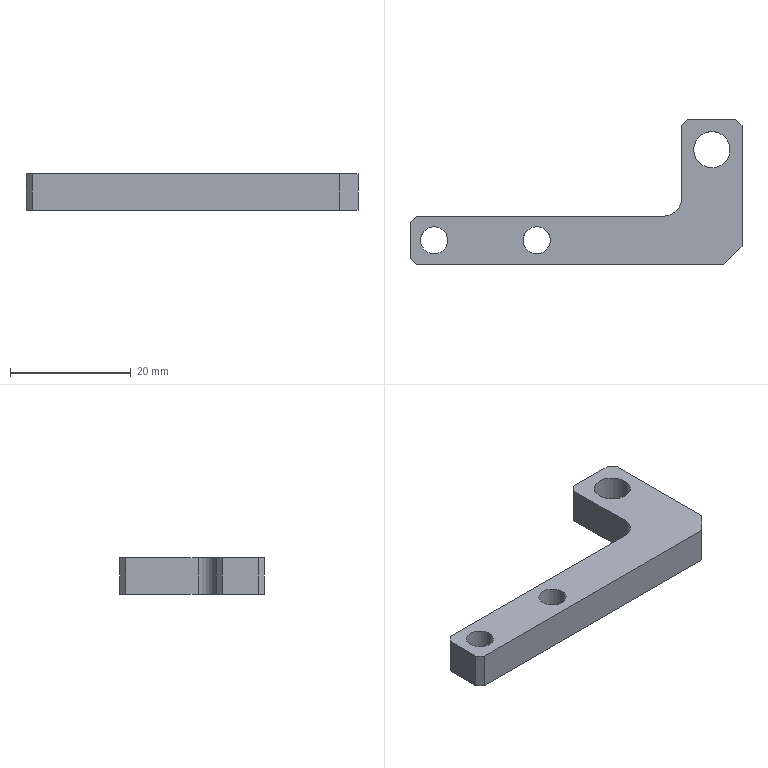Part | SolidWorks | features Chamfer 2, Extrusion 1, Fillet 1 | 1 solid | 20 faces | box 55 x 24 x 6 mm | volume 3212 mm3 | plane 13 | cylinder 7 | commonest cylinder face diameters 4.5 x4 6 x3
STEP:
#1=CARTESIAN_POINT('',(-8.,19.,3.));
#2=VERTEX_POINT('',#1);
#3=CARTESIAN_POINT('',(-2.,19.,3.));
#4=VERTEX_POINT('',#3);
#5=CARTESIAN_POINT('',(-5.,19.,3.));
#6=DIRECTION('',(0.,0.,1.));
#7=DIRECTION('',(1.,0.,0.));
#8=AXIS2_PLACEMENT_3D('',#5,#6,#7);
#9=CIRCLE('',#8,3.);
#10=EDGE_CURVE('',#2,#4,#9,.T.);
#11=ORIENTED_EDGE('',*,*,#10,.T.);
#12=CARTESIAN_POINT('',(-2.,19.,-3.));
#13=VERTEX_POINT('',#12);
#14=CARTESIAN_POINT('',(-2.,19.,3.));
#15=DIRECTION('',(0.,0.,-1.));
#16=VECTOR('',#15,1000.);
#17=LINE('',#14,#16);
#18=EDGE_CURVE('',#4,#13,#17,.T.);
#19=ORIENTED_EDGE('',*,*,#18,.T.);
#20=CARTESIAN_POINT('',(-8.,19.,-3.));
#21=VERTEX_POINT('',#20);
#22=CARTESIAN_POINT('',(-5.,19.,-3.));
#23=DIRECTION('',(0.,0.,1.));
#24=DIRECTION('',(1.,0.,0.));
#25=AXIS2_PLACEMENT_3D('',#22,#23,#24);
#26=CIRCLE('',#25,3.);
#27=EDGE_CURVE('',#21,#13,#26,.T.);
#28=ORIENTED_EDGE('',*,*,#27,.F.);
#29=CARTESIAN_POINT('',(-8.,19.,3.));
#30=DIRECTION('',(0.,0.,-1.));
#31=VECTOR('',#30,1000.);
#32=LINE('',#29,#31);
#33=EDGE_CURVE('',#2,#21,#32,.T.);
#34=ORIENTED_EDGE('',*,*,#33,.F.);
#35=EDGE_LOOP('',(#11,#19,#28,#34));
#36=FACE_OUTER_BOUND('',#35,.T.);
#37=CARTESIAN_POINT('',(-5.,19.,3.));
#38=DIRECTION('',(0.,0.,-1.));
#39=DIRECTION('',(-1.,0.,0.));
#40=AXIS2_PLACEMENT_3D('',#37,#38,#39);
#41=CYLINDRICAL_SURFACE('',#40,3.);
#42=ADVANCED_FACE('',(#36),#41,.F.);
#43=CARTESIAN_POINT('',(-36.25,4.,3.));
#44=VERTEX_POINT('',#43);
#45=CARTESIAN_POINT('',(-31.75,4.,3.));
#46=VERTEX_POINT('',#45);
#47=CARTESIAN_POINT('',(-34.,4.,3.));
#48=DIRECTION('',(0.,0.,1.));
#49=DIRECTION('',(1.,0.,0.));
#50=AXIS2_PLACEMENT_3D('',#47,#48,#49);
#51=CIRCLE('',#50,2.25);
#52=EDGE_CURVE('',#44,#46,#51,.T.);
#53=ORIENTED_EDGE('',*,*,#52,.T.);
#54=CARTESIAN_POINT('',(-31.75,4.,-3.));
#55=VERTEX_POINT('',#54);
#56=CARTESIAN_POINT('',(-31.75,4.,3.));
#57=DIRECTION('',(0.,0.,-1.));
#58=VECTOR('',#57,1000.);
#59=LINE('',#56,#58);
#60=EDGE_CURVE('',#46,#55,#59,.T.);
#61=ORIENTED_EDGE('',*,*,#60,.T.);
#62=CARTESIAN_POINT('',(-36.25,4.,-3.));
#63=VERTEX_POINT('',#62);
#64=CARTESIAN_POINT('',(-34.,4.,-3.));
#65=DIRECTION('',(0.,0.,1.));
#66=DIRECTION('',(1.,0.,0.));
#67=AXIS2_PLACEMENT_3D('',#64,#65,#66);
#68=CIRCLE('',#67,2.25);
#69=EDGE_CURVE('',#63,#55,#68,.T.);
#70=ORIENTED_EDGE('',*,*,#69,.F.);
#71=CARTESIAN_POINT('',(-36.25,4.,3.));
#72=DIRECTION('',(0.,0.,-1.));
#73=VECTOR('',#72,1000.);
#74=LINE('',#71,#73);
#75=EDGE_CURVE('',#44,#63,#74,.T.);
#76=ORIENTED_EDGE('',*,*,#75,.F.);
#77=EDGE_LOOP('',(#53,#61,#70,#76));
#78=FACE_OUTER_BOUND('',#77,.T.);
#79=CARTESIAN_POINT('',(-34.,4.,3.));
#80=DIRECTION('',(0.,0.,-1.));
#81=DIRECTION('',(-1.,0.,0.));
#82=AXIS2_PLACEMENT_3D('',#79,#80,#81);
#83=CYLINDRICAL_SURFACE('',#82,2.25);
#84=ADVANCED_FACE('',(#78),#83,.F.);
#85=CARTESIAN_POINT('',(-53.25,4.,3.));
#86=VERTEX_POINT('',#85);
#87=CARTESIAN_POINT('',(-48.75,4.,3.));
#88=VERTEX_POINT('',#87);
#89=CARTESIAN_POINT('',(-51.,4.,3.));
#90=DIRECTION('',(0.,0.,1.));
#91=DIRECTION('',(1.,0.,0.));
#92=AXIS2_PLACEMENT_3D('',#89,#90,#91);
#93=CIRCLE('',#92,2.25);
#94=EDGE_CURVE('',#86,#88,#93,.T.);
#95=ORIENTED_EDGE('',*,*,#94,.T.);
#96=CARTESIAN_POINT('',(-48.75,4.,-3.));
#97=VERTEX_POINT('',#96);
#98=CARTESIAN_POINT('',(-48.75,4.,3.));
#99=DIRECTION('',(0.,0.,-1.));
#100=VECTOR('',#99,1000.);
#101=LINE('',#98,#100);
#102=EDGE_CURVE('',#88,#97,#101,.T.);
#103=ORIENTED_EDGE('',*,*,#102,.T.);
#104=CARTESIAN_POINT('',(-53.25,4.,-3.));
#105=VERTEX_POINT('',#104);
#106=CARTESIAN_POINT('',(-51.,4.,-3.));
#107=DIRECTION('',(0.,0.,1.));
#108=DIRECTION('',(1.,0.,0.));
#109=AXIS2_PLACEMENT_3D('',#106,#107,#108);
#110=CIRCLE('',#109,2.25);
#111=EDGE_CURVE('',#105,#97,#110,.T.);
#112=ORIENTED_EDGE('',*,*,#111,.F.);
#113=CARTESIAN_POINT('',(-53.25,4.,3.));
#114=DIRECTION('',(0.,0.,-1.));
#115=VECTOR('',#114,1000.);
#116=LINE('',#113,#115);
#117=EDGE_CURVE('',#86,#105,#116,.T.);
#118=ORIENTED_EDGE('',*,*,#117,.F.);
#119=EDGE_LOOP('',(#95,#103,#112,#118));
#120=FACE_OUTER_BOUND('',#119,.T.);
#121=CARTESIAN_POINT('',(-51.,4.,3.));
#122=DIRECTION('',(0.,0.,-1.));
#123=DIRECTION('',(-1.,0.,0.));
#124=AXIS2_PLACEMENT_3D('',#121,#122,#123);
#125=CYLINDRICAL_SURFACE('',#124,2.25);
#126=ADVANCED_FACE('',(#120),#125,.F.);
#127=ORIENTED_EDGE('',*,*,#52,.F.);
#128=CARTESIAN_POINT('',(-34.,4.,3.));
#129=DIRECTION('',(0.,0.,1.));
#130=DIRECTION('',(1.,0.,0.));
#131=AXIS2_PLACEMENT_3D('',#128,#129,#130);
#132=CIRCLE('',#131,2.25);
#133=EDGE_CURVE('',#46,#44,#132,.T.);
#134=ORIENTED_EDGE('',*,*,#133,.F.);
#135=EDGE_LOOP('',(#127,#134));
#136=FACE_BOUND('',#135,.T.);
#137=CARTESIAN_POINT('',(-55.,7.,3.));
#138=VERTEX_POINT('',#137);
#139=CARTESIAN_POINT('',(-55.,1.,3.));
#140=VERTEX_POINT('',#139);
#141=CARTESIAN_POINT('',(-55.,0.,3.));
#142=DIRECTION('',(0.,-1.,0.));
#143=VECTOR('',#142,1000.);
#144=LINE('',#141,#143);
#145=EDGE_CURVE('',#138,#140,#144,.T.);
#146=ORIENTED_EDGE('',*,*,#145,.T.);
#147=CARTESIAN_POINT('',(-54.,0.,3.));
#148=VERTEX_POINT('',#147);
#149=CARTESIAN_POINT('',(-39.,-15.,3.));
#150=DIRECTION('',(0.7071,-0.7071,0.));
#151=VECTOR('',#150,1000.);
#152=LINE('',#149,#151);
#153=EDGE_CURVE('',#140,#148,#152,.T.);
#154=ORIENTED_EDGE('',*,*,#153,.T.);
#155=CARTESIAN_POINT('',(-3.,0.,3.));
#156=VERTEX_POINT('',#155);
#157=CARTESIAN_POINT('',(0.,0.,3.));
#158=DIRECTION('',(1.,0.,0.));
#159=VECTOR('',#158,1000.);
#160=LINE('',#157,#159);
#161=EDGE_CURVE('',#148,#156,#160,.T.);
#162=ORIENTED_EDGE('',*,*,#161,.T.);
#163=CARTESIAN_POINT('',(0.,3.,3.));
#164=VERTEX_POINT('',#163);
#165=CARTESIAN_POINT('',(10.5,13.5,3.));
#166=DIRECTION('',(0.7071,0.7071,0.));
#167=VECTOR('',#166,1000.);
#168=LINE('',#165,#167);
#169=EDGE_CURVE('',#156,#164,#168,.T.);
#170=ORIENTED_EDGE('',*,*,#169,.T.);
#171=CARTESIAN_POINT('',(0.,23.,3.));
#172=VERTEX_POINT('',#171);
#173=CARTESIAN_POINT('',(0.,0.,3.));
#174=DIRECTION('',(0.,1.,0.));
#175=VECTOR('',#174,1000.);
#176=LINE('',#173,#175);
#177=EDGE_CURVE('',#164,#172,#176,.T.);
#178=ORIENTED_EDGE('',*,*,#177,.T.);
#179=CARTESIAN_POINT('',(-1.,24.,3.));
#180=VERTEX_POINT('',#179);
#181=CARTESIAN_POINT('',(-0.5,23.5,3.));
#182=DIRECTION('',(-0.7071,0.7071,0.));
#183=VECTOR('',#182,1000.);
#184=LINE('',#181,#183);
#185=EDGE_CURVE('',#172,#180,#184,.T.);
#186=ORIENTED_EDGE('',*,*,#185,.T.);
#187=CARTESIAN_POINT('',(-9.,24.,3.));
#188=VERTEX_POINT('',#187);
#189=CARTESIAN_POINT('',(0.,24.,3.));
#190=DIRECTION('',(-1.,0.,0.));
#191=VECTOR('',#190,1000.);
#192=LINE('',#189,#191);
#193=EDGE_CURVE('',#180,#188,#192,.T.);
#194=ORIENTED_EDGE('',*,*,#193,.T.);
#195=CARTESIAN_POINT('',(-10.,23.,3.));
#196=VERTEX_POINT('',#195);
#197=CARTESIAN_POINT('',(-4.5,28.5,3.));
#198=DIRECTION('',(-0.7071,-0.7071,0.));
#199=VECTOR('',#198,1000.);
#200=LINE('',#197,#199);
#201=EDGE_CURVE('',#188,#196,#200,.T.);
#202=ORIENTED_EDGE('',*,*,#201,.T.);
#203=CARTESIAN_POINT('',(-10.,11.,3.));
#204=VERTEX_POINT('',#203);
#205=CARTESIAN_POINT('',(-10.,24.,3.));
#206=DIRECTION('',(0.,-1.,0.));
#207=VECTOR('',#206,1000.);
#208=LINE('',#205,#207);
#209=EDGE_CURVE('',#196,#204,#208,.T.);
#210=ORIENTED_EDGE('',*,*,#209,.T.);
#211=CARTESIAN_POINT('',(-13.,8.,3.));
#212=VERTEX_POINT('',#211);
#213=CARTESIAN_POINT('',(-13.,11.,3.));
#214=DIRECTION('',(0.,0.,-1.));
#215=DIRECTION('',(1.,0.,0.));
#216=AXIS2_PLACEMENT_3D('',#213,#214,#215);
#217=CIRCLE('',#216,3.);
#218=EDGE_CURVE('',#204,#212,#217,.T.);
#219=ORIENTED_EDGE('',*,*,#218,.T.);
#220=CARTESIAN_POINT('',(-54.,8.,3.));
#221=VERTEX_POINT('',#220);
#222=CARTESIAN_POINT('',(-55.,8.,3.));
#223=DIRECTION('',(-1.,0.,0.));
#224=VECTOR('',#223,1000.);
#225=LINE('',#222,#224);
#226=EDGE_CURVE('',#212,#221,#225,.T.);
#227=ORIENTED_EDGE('',*,*,#226,.T.);
#228=CARTESIAN_POINT('',(-19.,43.,3.));
#229=DIRECTION('',(-0.7071,-0.7071,0.));
#230=VECTOR('',#229,1000.);
#231=LINE('',#228,#230);
#232=EDGE_CURVE('',#221,#138,#231,.T.);
#233=ORIENTED_EDGE('',*,*,#232,.T.);
#234=EDGE_LOOP('',(#146,#154,#162,#170,#178,#186,#194,#202,#210,#219,#227,#233));
#235=FACE_OUTER_BOUND('',#234,.T.);
#236=ORIENTED_EDGE('',*,*,#94,.F.);
#237=CARTESIAN_POINT('',(-51.,4.,3.));
#238=DIRECTION('',(0.,0.,1.));
#239=DIRECTION('',(1.,0.,0.));
#240=AXIS2_PLACEMENT_3D('',#237,#238,#239);
#241=CIRCLE('',#240,2.25);
#242=EDGE_CURVE('',#88,#86,#241,.T.);
#243=ORIENTED_EDGE('',*,*,#242,.F.);
#244=EDGE_LOOP('',(#236,#243));
#245=FACE_BOUND('',#244,.T.);
#246=ORIENTED_EDGE('',*,*,#10,.F.);
#247=CARTESIAN_POINT('',(-5.,19.,3.));
#248=DIRECTION('',(0.,0.,1.));
#249=DIRECTION('',(1.,0.,0.));
#250=AXIS2_PLACEMENT_3D('',#247,#248,#249);
#251=CIRCLE('',#250,3.);
#252=EDGE_CURVE('',#4,#2,#251,.T.);
#253=ORIENTED_EDGE('',*,*,#252,.F.);
#254=EDGE_LOOP('',(#246,#253));
#255=FACE_BOUND('',#254,.T.);
#256=CARTESIAN_POINT('',(0.,24.,3.));
#257=DIRECTION('',(0.,0.,1.));
#258=DIRECTION('',(1.,0.,0.));
#259=AXIS2_PLACEMENT_3D('',#256,#257,#258);
#260=PLANE('',#259);
#261=ADVANCED_FACE('',(#136,#235,#245,#255),#260,.T.);
#262=ORIENTED_EDGE('',*,*,#69,.T.);
#263=CARTESIAN_POINT('',(-34.,4.,-3.));
#264=DIRECTION('',(0.,0.,1.));
#265=DIRECTION('',(1.,0.,0.));
#266=AXIS2_PLACEMENT_3D('',#263,#264,#265);
#267=CIRCLE('',#266,2.25);
#268=EDGE_CURVE('',#55,#63,#267,.T.);
#269=ORIENTED_EDGE('',*,*,#268,.T.);
#270=EDGE_LOOP('',(#262,#269));
#271=FACE_BOUND('',#270,.T.);
#272=CARTESIAN_POINT('',(-54.,0.,-3.));
#273=VERTEX_POINT('',#272);
#274=CARTESIAN_POINT('',(-3.,0.,-3.));
#275=VERTEX_POINT('',#274);
#276=CARTESIAN_POINT('',(0.,0.,-3.));
#277=DIRECTION('',(1.,0.,0.));
#278=VECTOR('',#277,1000.);
#279=LINE('',#276,#278);
#280=EDGE_CURVE('',#273,#275,#279,.T.);
#281=ORIENTED_EDGE('',*,*,#280,.F.);
#282=CARTESIAN_POINT('',(-55.,1.,-3.));
#283=VERTEX_POINT('',#282);
#284=CARTESIAN_POINT('',(-54.,0.,-3.));
#285=DIRECTION('',(-0.7071,0.7071,0.));
#286=VECTOR('',#285,1000.);
#287=LINE('',#284,#286);
#288=EDGE_CURVE('',#273,#283,#287,.T.);
#289=ORIENTED_EDGE('',*,*,#288,.T.);
#290=CARTESIAN_POINT('',(-55.,7.,-3.));
#291=VERTEX_POINT('',#290);
#292=CARTESIAN_POINT('',(-55.,0.,-3.));
#293=DIRECTION('',(0.,-1.,0.));
#294=VECTOR('',#293,1000.);
#295=LINE('',#292,#294);
#296=EDGE_CURVE('',#291,#283,#295,.T.);
#297=ORIENTED_EDGE('',*,*,#296,.F.);
#298=CARTESIAN_POINT('',(-54.,8.,-3.));
#299=VERTEX_POINT('',#298);
#300=CARTESIAN_POINT('',(-55.,7.,-3.));
#301=DIRECTION('',(0.7071,0.7071,0.));
#302=VECTOR('',#301,1000.);
#303=LINE('',#300,#302);
#304=EDGE_CURVE('',#291,#299,#303,.T.);
#305=ORIENTED_EDGE('',*,*,#304,.T.);
#306=CARTESIAN_POINT('',(-13.,8.,-3.));
#307=VERTEX_POINT('',#306);
#308=CARTESIAN_POINT('',(-55.,8.,-3.));
#309=DIRECTION('',(-1.,0.,0.));
#310=VECTOR('',#309,1000.);
#311=LINE('',#308,#310);
#312=EDGE_CURVE('',#307,#299,#311,.T.);
#313=ORIENTED_EDGE('',*,*,#312,.F.);
#314=CARTESIAN_POINT('',(-10.,11.,-3.));
#315=VERTEX_POINT('',#314);
#316=CARTESIAN_POINT('',(-13.,11.,-3.));
#317=DIRECTION('',(0.,0.,1.));
#318=DIRECTION('',(1.,0.,0.));
#319=AXIS2_PLACEMENT_3D('',#316,#317,#318);
#320=CIRCLE('',#319,3.);
#321=EDGE_CURVE('',#307,#315,#320,.T.);
#322=ORIENTED_EDGE('',*,*,#321,.T.);
#323=CARTESIAN_POINT('',(-10.,23.,-3.));
#324=VERTEX_POINT('',#323);
#325=CARTESIAN_POINT('',(-10.,24.,-3.));
#326=DIRECTION('',(0.,-1.,0.));
#327=VECTOR('',#326,1000.);
#328=LINE('',#325,#327);
#329=EDGE_CURVE('',#324,#315,#328,.T.);
#330=ORIENTED_EDGE('',*,*,#329,.F.);
#331=CARTESIAN_POINT('',(-9.,24.,-3.));
#332=VERTEX_POINT('',#331);
#333=CARTESIAN_POINT('',(-10.,23.,-3.));
#334=DIRECTION('',(0.7071,0.7071,0.));
#335=VECTOR('',#334,1000.);
#336=LINE('',#333,#335);
#337=EDGE_CURVE('',#324,#332,#336,.T.);
#338=ORIENTED_EDGE('',*,*,#337,.T.);
#339=CARTESIAN_POINT('',(-1.,24.,-3.));
#340=VERTEX_POINT('',#339);
#341=CARTESIAN_POINT('',(0.,24.,-3.));
#342=DIRECTION('',(-1.,0.,0.));
#343=VECTOR('',#342,1000.);
#344=LINE('',#341,#343);
#345=EDGE_CURVE('',#340,#332,#344,.T.);
#346=ORIENTED_EDGE('',*,*,#345,.F.);
#347=CARTESIAN_POINT('',(0.,23.,-3.));
#348=VERTEX_POINT('',#347);
#349=CARTESIAN_POINT('',(-1.,24.,-3.));
#350=DIRECTION('',(0.7071,-0.7071,0.));
#351=VECTOR('',#350,1000.);
#352=LINE('',#349,#351);
#353=EDGE_CURVE('',#340,#348,#352,.T.);
#354=ORIENTED_EDGE('',*,*,#353,.T.);
#355=CARTESIAN_POINT('',(0.,3.,-3.));
#356=VERTEX_POINT('',#355);
#357=CARTESIAN_POINT('',(0.,0.,-3.));
#358=DIRECTION('',(0.,1.,0.));
#359=VECTOR('',#358,1000.);
#360=LINE('',#357,#359);
#361=EDGE_CURVE('',#356,#348,#360,.T.);
#362=ORIENTED_EDGE('',*,*,#361,.F.);
#363=CARTESIAN_POINT('',(0.,3.,-3.));
#364=DIRECTION('',(-0.7071,-0.7071,0.));
#365=VECTOR('',#364,1000.);
#366=LINE('',#363,#365);
#367=EDGE_CURVE('',#356,#275,#366,.T.);
#368=ORIENTED_EDGE('',*,*,#367,.T.);
#369=EDGE_LOOP('',(#281,#289,#297,#305,#313,#322,#330,#338,#346,#354,#362,#368));
#370=FACE_OUTER_BOUND('',#369,.T.);
#371=ORIENTED_EDGE('',*,*,#111,.T.);
#372=CARTESIAN_POINT('',(-51.,4.,-3.));
#373=DIRECTION('',(0.,0.,1.));
#374=DIRECTION('',(1.,0.,0.));
#375=AXIS2_PLACEMENT_3D('',#372,#373,#374);
#376=CIRCLE('',#375,2.25);
#377=EDGE_CURVE('',#97,#105,#376,.T.);
#378=ORIENTED_EDGE('',*,*,#377,.T.);
#379=EDGE_LOOP('',(#371,#378));
#380=FACE_BOUND('',#379,.T.);
#381=ORIENTED_EDGE('',*,*,#27,.T.);
#382=CARTESIAN_POINT('',(-5.,19.,-3.));
#383=DIRECTION('',(0.,0.,1.));
#384=DIRECTION('',(1.,0.,0.));
#385=AXIS2_PLACEMENT_3D('',#382,#383,#384);
#386=CIRCLE('',#385,3.);
#387=EDGE_CURVE('',#13,#21,#386,.T.);
#388=ORIENTED_EDGE('',*,*,#387,.T.);
#389=EDGE_LOOP('',(#381,#388));
#390=FACE_BOUND('',#389,.T.);
#391=CARTESIAN_POINT('',(0.,24.,-3.));
#392=DIRECTION('',(0.,0.,1.));
#393=DIRECTION('',(1.,0.,0.));
#394=AXIS2_PLACEMENT_3D('',#391,#392,#393);
#395=PLANE('',#394);
#396=ADVANCED_FACE('',(#271,#370,#380,#390),#395,.F.);
#397=ORIENTED_EDGE('',*,*,#361,.T.);
#398=CARTESIAN_POINT('',(0.,23.,3.));
#399=DIRECTION('',(0.,0.,1.));
#400=VECTOR('',#399,1000.);
#401=LINE('',#398,#400);
#402=EDGE_CURVE('',#348,#172,#401,.T.);
#403=ORIENTED_EDGE('',*,*,#402,.T.);
#404=ORIENTED_EDGE('',*,*,#177,.F.);
#405=CARTESIAN_POINT('',(0.,3.,3.));
#406=DIRECTION('',(0.,0.,-1.));
#407=VECTOR('',#406,1000.);
#408=LINE('',#405,#407);
#409=EDGE_CURVE('',#164,#356,#408,.T.);
#410=ORIENTED_EDGE('',*,*,#409,.T.);
#411=EDGE_LOOP('',(#397,#403,#404,#410));
#412=FACE_OUTER_BOUND('',#411,.T.);
#413=CARTESIAN_POINT('',(0.,0.,3.));
#414=DIRECTION('',(-1.,0.,0.));
#415=DIRECTION('',(0.,0.,1.));
#416=AXIS2_PLACEMENT_3D('',#413,#414,#415);
#417=PLANE('',#416);
#418=ADVANCED_FACE('',(#412),#417,.F.);
#419=ORIENTED_EDGE('',*,*,#345,.T.);
#420=CARTESIAN_POINT('',(-9.,24.,3.));
#421=DIRECTION('',(0.,0.,1.));
#422=VECTOR('',#421,1000.);
#423=LINE('',#420,#422);
#424=EDGE_CURVE('',#332,#188,#423,.T.);
#425=ORIENTED_EDGE('',*,*,#424,.T.);
#426=ORIENTED_EDGE('',*,*,#193,.F.);
#427=CARTESIAN_POINT('',(-1.,24.,3.));
#428=DIRECTION('',(0.,0.,-1.));
#429=VECTOR('',#428,1000.);
#430=LINE('',#427,#429);
#431=EDGE_CURVE('',#180,#340,#430,.T.);
#432=ORIENTED_EDGE('',*,*,#431,.T.);
#433=EDGE_LOOP('',(#419,#425,#426,#432));
#434=FACE_OUTER_BOUND('',#433,.T.);
#435=CARTESIAN_POINT('',(0.,24.,3.));
#436=DIRECTION('',(0.,-1.,0.));
#437=DIRECTION('',(0.,0.,-1.));
#438=AXIS2_PLACEMENT_3D('',#435,#436,#437);
#439=PLANE('',#438);
#440=ADVANCED_FACE('',(#434),#439,.F.);
#441=ORIENTED_EDGE('',*,*,#209,.F.);
#442=CARTESIAN_POINT('',(-10.,23.,3.));
#443=DIRECTION('',(0.,0.,-1.));
#444=VECTOR('',#443,1000.);
#445=LINE('',#442,#444);
#446=EDGE_CURVE('',#196,#324,#445,.T.);
#447=ORIENTED_EDGE('',*,*,#446,.T.);
#448=ORIENTED_EDGE('',*,*,#329,.T.);
#449=CARTESIAN_POINT('',(-10.,11.,3.));
#450=DIRECTION('',(0.,0.,1.));
#451=VECTOR('',#450,1000.);
#452=LINE('',#449,#451);
#453=EDGE_CURVE('',#315,#204,#452,.T.);
#454=ORIENTED_EDGE('',*,*,#453,.T.);
#455=EDGE_LOOP('',(#441,#447,#448,#454));
#456=FACE_OUTER_BOUND('',#455,.T.);
#457=CARTESIAN_POINT('',(-10.,24.,3.));
#458=DIRECTION('',(1.,0.,0.));
#459=DIRECTION('',(0.,1.,0.));
#460=AXIS2_PLACEMENT_3D('',#457,#458,#459);
#461=PLANE('',#460);
#462=ADVANCED_FACE('',(#456),#461,.F.);
#463=ORIENTED_EDGE('',*,*,#312,.T.);
#464=CARTESIAN_POINT('',(-54.,8.,3.));
#465=DIRECTION('',(0.,0.,1.));
#466=VECTOR('',#465,1000.);
#467=LINE('',#464,#466);
#468=EDGE_CURVE('',#299,#221,#467,.T.);
#469=ORIENTED_EDGE('',*,*,#468,.T.);
#470=ORIENTED_EDGE('',*,*,#226,.F.);
#471=CARTESIAN_POINT('',(-13.,8.,-3.));
#472=DIRECTION('',(0.,0.,-1.));
#473=VECTOR('',#472,1000.);
#474=LINE('',#471,#473);
#475=EDGE_CURVE('',#212,#307,#474,.T.);
#476=ORIENTED_EDGE('',*,*,#475,.T.);
#477=EDGE_LOOP('',(#463,#469,#470,#476));
#478=FACE_OUTER_BOUND('',#477,.T.);
#479=CARTESIAN_POINT('',(-55.,8.,3.));
#480=DIRECTION('',(0.,-1.,0.));
#481=DIRECTION('',(0.,0.,-1.));
#482=AXIS2_PLACEMENT_3D('',#479,#480,#481);
#483=PLANE('',#482);
#484=ADVANCED_FACE('',(#478),#483,.F.);
#485=ORIENTED_EDGE('',*,*,#296,.T.);
#486=CARTESIAN_POINT('',(-55.,1.,3.));
#487=DIRECTION('',(0.,0.,1.));
#488=VECTOR('',#487,1000.);
#489=LINE('',#486,#488);
#490=EDGE_CURVE('',#283,#140,#489,.T.);
#491=ORIENTED_EDGE('',*,*,#490,.T.);
#492=ORIENTED_EDGE('',*,*,#145,.F.);
#493=CARTESIAN_POINT('',(-55.,7.,3.));
#494=DIRECTION('',(0.,0.,-1.));
#495=VECTOR('',#494,1000.);
#496=LINE('',#493,#495);
#497=EDGE_CURVE('',#138,#291,#496,.T.);
#498=ORIENTED_EDGE('',*,*,#497,.T.);
#499=EDGE_LOOP('',(#485,#491,#492,#498));
#500=FACE_OUTER_BOUND('',#499,.T.);
#501=CARTESIAN_POINT('',(-55.,0.,3.));
#502=DIRECTION('',(1.,0.,0.));
#503=DIRECTION('',(0.,0.,-1.));
#504=AXIS2_PLACEMENT_3D('',#501,#502,#503);
#505=PLANE('',#504);
#506=ADVANCED_FACE('',(#500),#505,.F.);
#507=ORIENTED_EDGE('',*,*,#161,.F.);
#508=CARTESIAN_POINT('',(-54.,0.,3.));
#509=DIRECTION('',(0.,0.,-1.));
#510=VECTOR('',#509,1000.);
#511=LINE('',#508,#510);
#512=EDGE_CURVE('',#148,#273,#511,.T.);
#513=ORIENTED_EDGE('',*,*,#512,.T.);
#514=ORIENTED_EDGE('',*,*,#280,.T.);
#515=CARTESIAN_POINT('',(-3.,0.,3.));
#516=DIRECTION('',(0.,0.,1.));
#517=VECTOR('',#516,1000.);
#518=LINE('',#515,#517);
#519=EDGE_CURVE('',#275,#156,#518,.T.);
#520=ORIENTED_EDGE('',*,*,#519,.T.);
#521=EDGE_LOOP('',(#507,#513,#514,#520));
#522=FACE_OUTER_BOUND('',#521,.T.);
#523=CARTESIAN_POINT('',(0.,0.,3.));
#524=DIRECTION('',(0.,1.,0.));
#525=DIRECTION('',(-1.,0.,0.));
#526=AXIS2_PLACEMENT_3D('',#523,#524,#525);
#527=PLANE('',#526);
#528=ADVANCED_FACE('',(#522),#527,.F.);
#529=ORIENTED_EDGE('',*,*,#102,.F.);
#530=ORIENTED_EDGE('',*,*,#242,.T.);
#531=ORIENTED_EDGE('',*,*,#117,.T.);
#532=ORIENTED_EDGE('',*,*,#377,.F.);
#533=EDGE_LOOP('',(#529,#530,#531,#532));
#534=FACE_OUTER_BOUND('',#533,.T.);
#535=CARTESIAN_POINT('',(-51.,4.,3.));
#536=DIRECTION('',(0.,0.,-1.));
#537=DIRECTION('',(-1.,0.,0.));
#538=AXIS2_PLACEMENT_3D('',#535,#536,#537);
#539=CYLINDRICAL_SURFACE('',#538,2.25);
#540=ADVANCED_FACE('',(#534),#539,.F.);
#541=ORIENTED_EDGE('',*,*,#60,.F.);
#542=ORIENTED_EDGE('',*,*,#133,.T.);
#543=ORIENTED_EDGE('',*,*,#75,.T.);
#544=ORIENTED_EDGE('',*,*,#268,.F.);
#545=EDGE_LOOP('',(#541,#542,#543,#544));
#546=FACE_OUTER_BOUND('',#545,.T.);
#547=CARTESIAN_POINT('',(-34.,4.,3.));
#548=DIRECTION('',(0.,0.,-1.));
#549=DIRECTION('',(-1.,0.,0.));
#550=AXIS2_PLACEMENT_3D('',#547,#548,#549);
#551=CYLINDRICAL_SURFACE('',#550,2.25);
#552=ADVANCED_FACE('',(#546),#551,.F.);
#553=ORIENTED_EDGE('',*,*,#18,.F.);
#554=ORIENTED_EDGE('',*,*,#252,.T.);
#555=ORIENTED_EDGE('',*,*,#33,.T.);
#556=ORIENTED_EDGE('',*,*,#387,.F.);
#557=EDGE_LOOP('',(#553,#554,#555,#556));
#558=FACE_OUTER_BOUND('',#557,.T.);
#559=CARTESIAN_POINT('',(-5.,19.,3.));
#560=DIRECTION('',(0.,0.,-1.));
#561=DIRECTION('',(-1.,0.,0.));
#562=AXIS2_PLACEMENT_3D('',#559,#560,#561);
#563=CYLINDRICAL_SURFACE('',#562,3.);
#564=ADVANCED_FACE('',(#558),#563,.F.);
#565=ORIENTED_EDGE('',*,*,#218,.F.);
#566=ORIENTED_EDGE('',*,*,#453,.F.);
#567=ORIENTED_EDGE('',*,*,#321,.F.);
#568=ORIENTED_EDGE('',*,*,#475,.F.);
#569=EDGE_LOOP('',(#565,#566,#567,#568));
#570=FACE_OUTER_BOUND('',#569,.T.);
#571=CARTESIAN_POINT('',(-13.,11.,3.));
#572=DIRECTION('',(0.,0.,1.));
#573=DIRECTION('',(1.,0.,0.));
#574=AXIS2_PLACEMENT_3D('',#571,#572,#573);
#575=CYLINDRICAL_SURFACE('',#574,3.);
#576=ADVANCED_FACE('',(#570),#575,.F.);
#577=ORIENTED_EDGE('',*,*,#169,.F.);
#578=ORIENTED_EDGE('',*,*,#519,.F.);
#579=ORIENTED_EDGE('',*,*,#367,.F.);
#580=ORIENTED_EDGE('',*,*,#409,.F.);
#581=EDGE_LOOP('',(#577,#578,#579,#580));
#582=FACE_OUTER_BOUND('',#581,.T.);
#583=CARTESIAN_POINT('',(0.,3.,3.));
#584=DIRECTION('',(-0.7071,0.7071,0.));
#585=DIRECTION('',(-0.7071,-0.7071,0.));
#586=AXIS2_PLACEMENT_3D('',#583,#584,#585);
#587=PLANE('',#586);
#588=ADVANCED_FACE('',(#582),#587,.F.);
#589=ORIENTED_EDGE('',*,*,#153,.F.);
#590=ORIENTED_EDGE('',*,*,#490,.F.);
#591=ORIENTED_EDGE('',*,*,#288,.F.);
#592=ORIENTED_EDGE('',*,*,#512,.F.);
#593=EDGE_LOOP('',(#589,#590,#591,#592));
#594=FACE_OUTER_BOUND('',#593,.T.);
#595=CARTESIAN_POINT('',(-54.,0.,3.));
#596=DIRECTION('',(0.7071,0.7071,0.));
#597=DIRECTION('',(-0.7071,0.7071,0.));
#598=AXIS2_PLACEMENT_3D('',#595,#596,#597);
#599=PLANE('',#598);
#600=ADVANCED_FACE('',(#594),#599,.F.);
#601=ORIENTED_EDGE('',*,*,#232,.F.);
#602=ORIENTED_EDGE('',*,*,#468,.F.);
#603=ORIENTED_EDGE('',*,*,#304,.F.);
#604=ORIENTED_EDGE('',*,*,#497,.F.);
#605=EDGE_LOOP('',(#601,#602,#603,#604));
#606=FACE_OUTER_BOUND('',#605,.T.);
#607=CARTESIAN_POINT('',(-55.,7.,3.));
#608=DIRECTION('',(0.7071,-0.7071,0.));
#609=DIRECTION('',(0.7071,0.7071,0.));
#610=AXIS2_PLACEMENT_3D('',#607,#608,#609);
#611=PLANE('',#610);
#612=ADVANCED_FACE('',(#606),#611,.F.);
#613=ORIENTED_EDGE('',*,*,#201,.F.);
#614=ORIENTED_EDGE('',*,*,#424,.F.);
#615=ORIENTED_EDGE('',*,*,#337,.F.);
#616=ORIENTED_EDGE('',*,*,#446,.F.);
#617=EDGE_LOOP('',(#613,#614,#615,#616));
#618=FACE_OUTER_BOUND('',#617,.T.);
#619=CARTESIAN_POINT('',(-10.,23.,3.));
#620=DIRECTION('',(0.7071,-0.7071,0.));
#621=DIRECTION('',(0.7071,0.7071,0.));
#622=AXIS2_PLACEMENT_3D('',#619,#620,#621);
#623=PLANE('',#622);
#624=ADVANCED_FACE('',(#618),#623,.F.);
#625=ORIENTED_EDGE('',*,*,#185,.F.);
#626=ORIENTED_EDGE('',*,*,#402,.F.);
#627=ORIENTED_EDGE('',*,*,#353,.F.);
#628=ORIENTED_EDGE('',*,*,#431,.F.);
#629=EDGE_LOOP('',(#625,#626,#627,#628));
#630=FACE_OUTER_BOUND('',#629,.T.);
#631=CARTESIAN_POINT('',(-1.,24.,3.));
#632=DIRECTION('',(-0.7071,-0.7071,0.));
#633=DIRECTION('',(0.7071,-0.7071,0.));
#634=AXIS2_PLACEMENT_3D('',#631,#632,#633);
#635=PLANE('',#634);
#636=ADVANCED_FACE('',(#630),#635,.F.);
#637=CLOSED_SHELL('',(#42,#84,#126,#261,#396,#418,#440,#462,#484,#506,#528,#540,#552,#564,#576,#588,#600,#612,#624,#636));
#638=MANIFOLD_SOLID_BREP('',#637);
#639=CARTESIAN_POINT('',(0.,0.,0.));
#640=DIRECTION('',(0.,0.,1.));
#641=DIRECTION('',(1.,0.,0.));
#642=AXIS2_PLACEMENT_3D('',#639,#640,#641);
#643=(LENGTH_UNIT()NAMED_UNIT(*)SI_UNIT(.MILLI.,.METRE.));
#644=UNCERTAINTY_MEASURE_WITH_UNIT(LENGTH_MEASURE(0.00001),#643,'','');
#645=(NAMED_UNIT(*)PLANE_ANGLE_UNIT()SI_UNIT($,.RADIAN.));
#646=(NAMED_UNIT(*)SI_UNIT($,.STERADIAN.)SOLID_ANGLE_UNIT());
#647=(GEOMETRIC_REPRESENTATION_CONTEXT(3)GLOBAL_UNCERTAINTY_ASSIGNED_CONTEXT((#644))GLOBAL_UNIT_ASSIGNED_CONTEXT((#643,#645,#646))REPRESENTATION_CONTEXT('',''));
#648=ADVANCED_BREP_SHAPE_REPRESENTATION('',(#638,#642),#647);